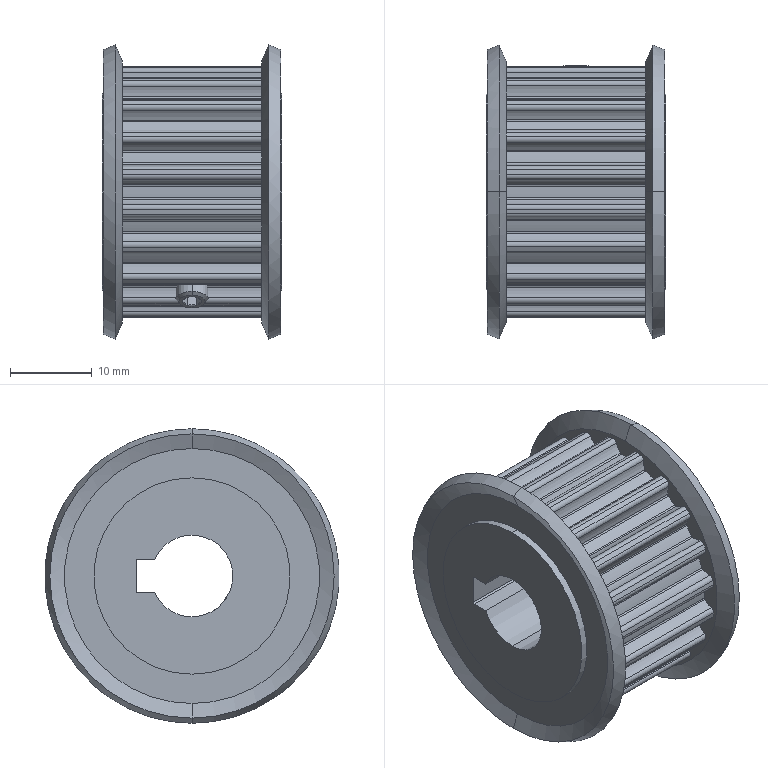Part | STEP file | HTPA20S5M150-A-NK10 | 3 solids | 262 faces | box 22 x 36 x 36 mm | volume 13148 mm3 | cylinder 201 | cone 34 | plane 27 | commonest cylinder face diameters 1.1 x53 0.5 x45 6.55 x43 27.33 x22 30.87 x21 3.242 x4